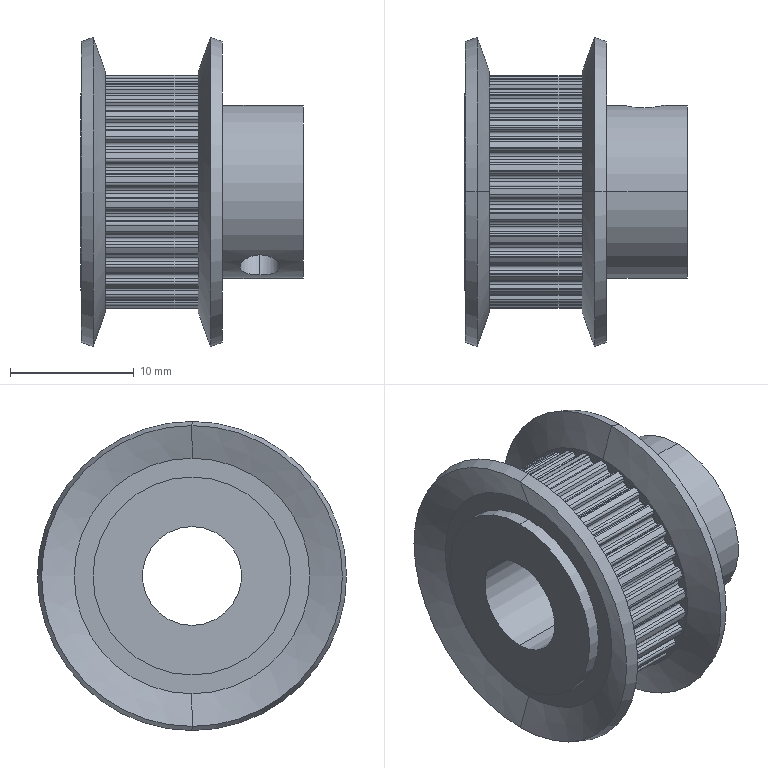Part | STEP file | ATP30MXL025-B-P8 | 1 solid | 296 faces | box 18 x 25 x 25 mm | volume 3402 mm3 | cylinder 217 | plane 67 | cone 12 | commonest cylinder face diameters 0.46 x72 0.6 x72 18.9 x31 17.62 x30 3.242 x4 16 x4